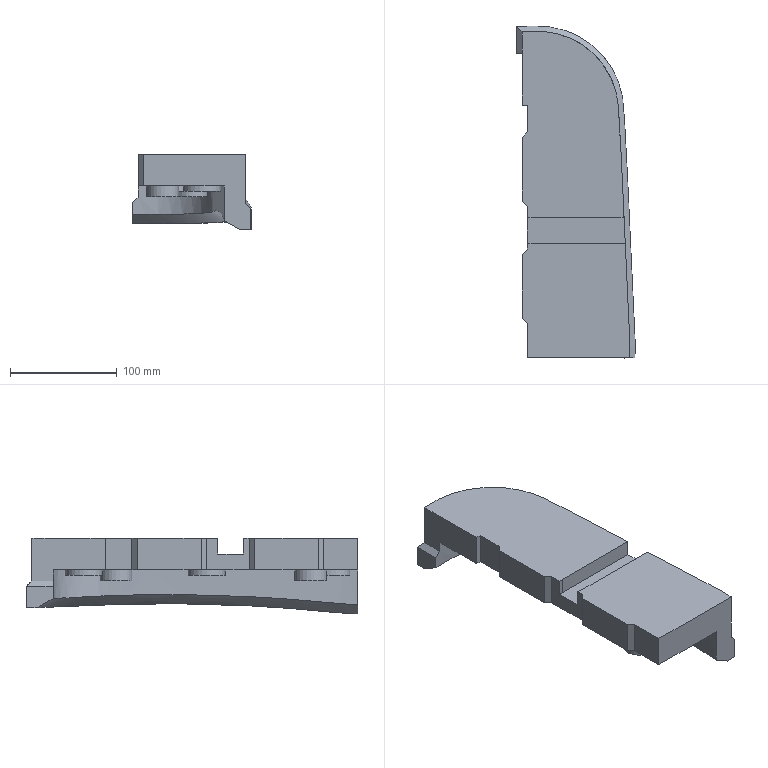Part | NX | features solid 2 | 1 solid | 38 faces | box 111.229 x 311.407 x 71.262 mm | volume 1074080 mm3 | plane 24 | spline 7 | cylinder 7 | commonest cylinder face diameters 35 x3 25 x2 30 x2